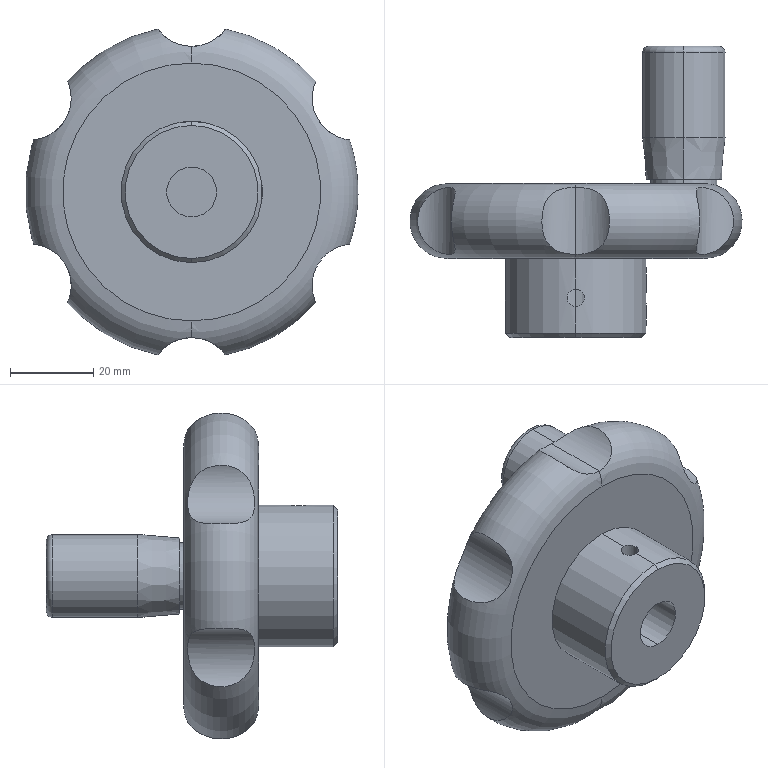Part | SolidWorks | features BaseBody 1 | 1 solid | 37 faces | box 80 x 70 x 78.333 mm | volume 98005 mm3 | cylinder 19 | cone 7 | plane 7 | torus 4 | commonest cylinder face diameters 20 x9 4.134 x4 12 x2 16 x2 34 x2